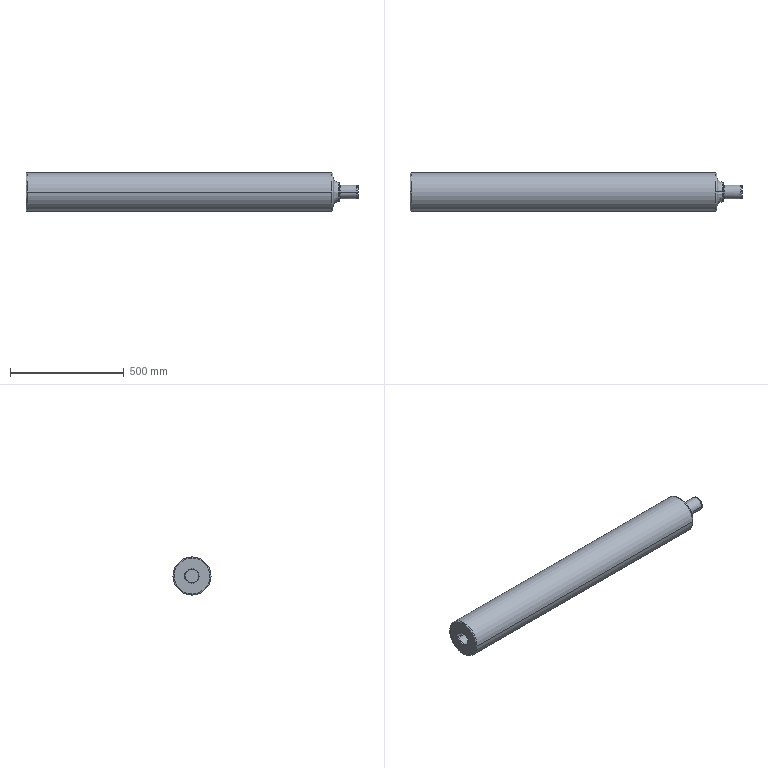Part | SolidWorks | features BaseBody 1 | 1 solid | 60 faces | box 1461 x 168 x 168 mm | volume 11688536 mm3 | cylinder 23 | cone 15 | plane 14 | spline 8 | commonest cylinder face diameters 60 x7 6 x4 7.95 x2 55.8 x2 72 x2 85 x2